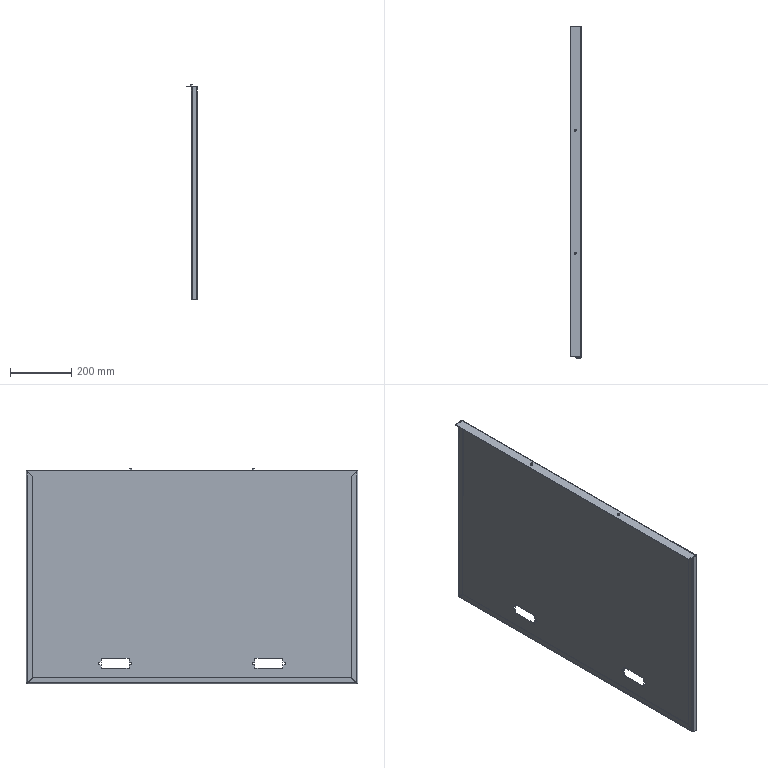Part | STEP file | HT-2 | 3 solids | 94 faces | box 35 x 1080 x 702 mm | volume 1298798 mm3 | plane 62 | cylinder 26 | spline 6 | commonest cylinder face diameters 3 x11 6 x11 8 x4